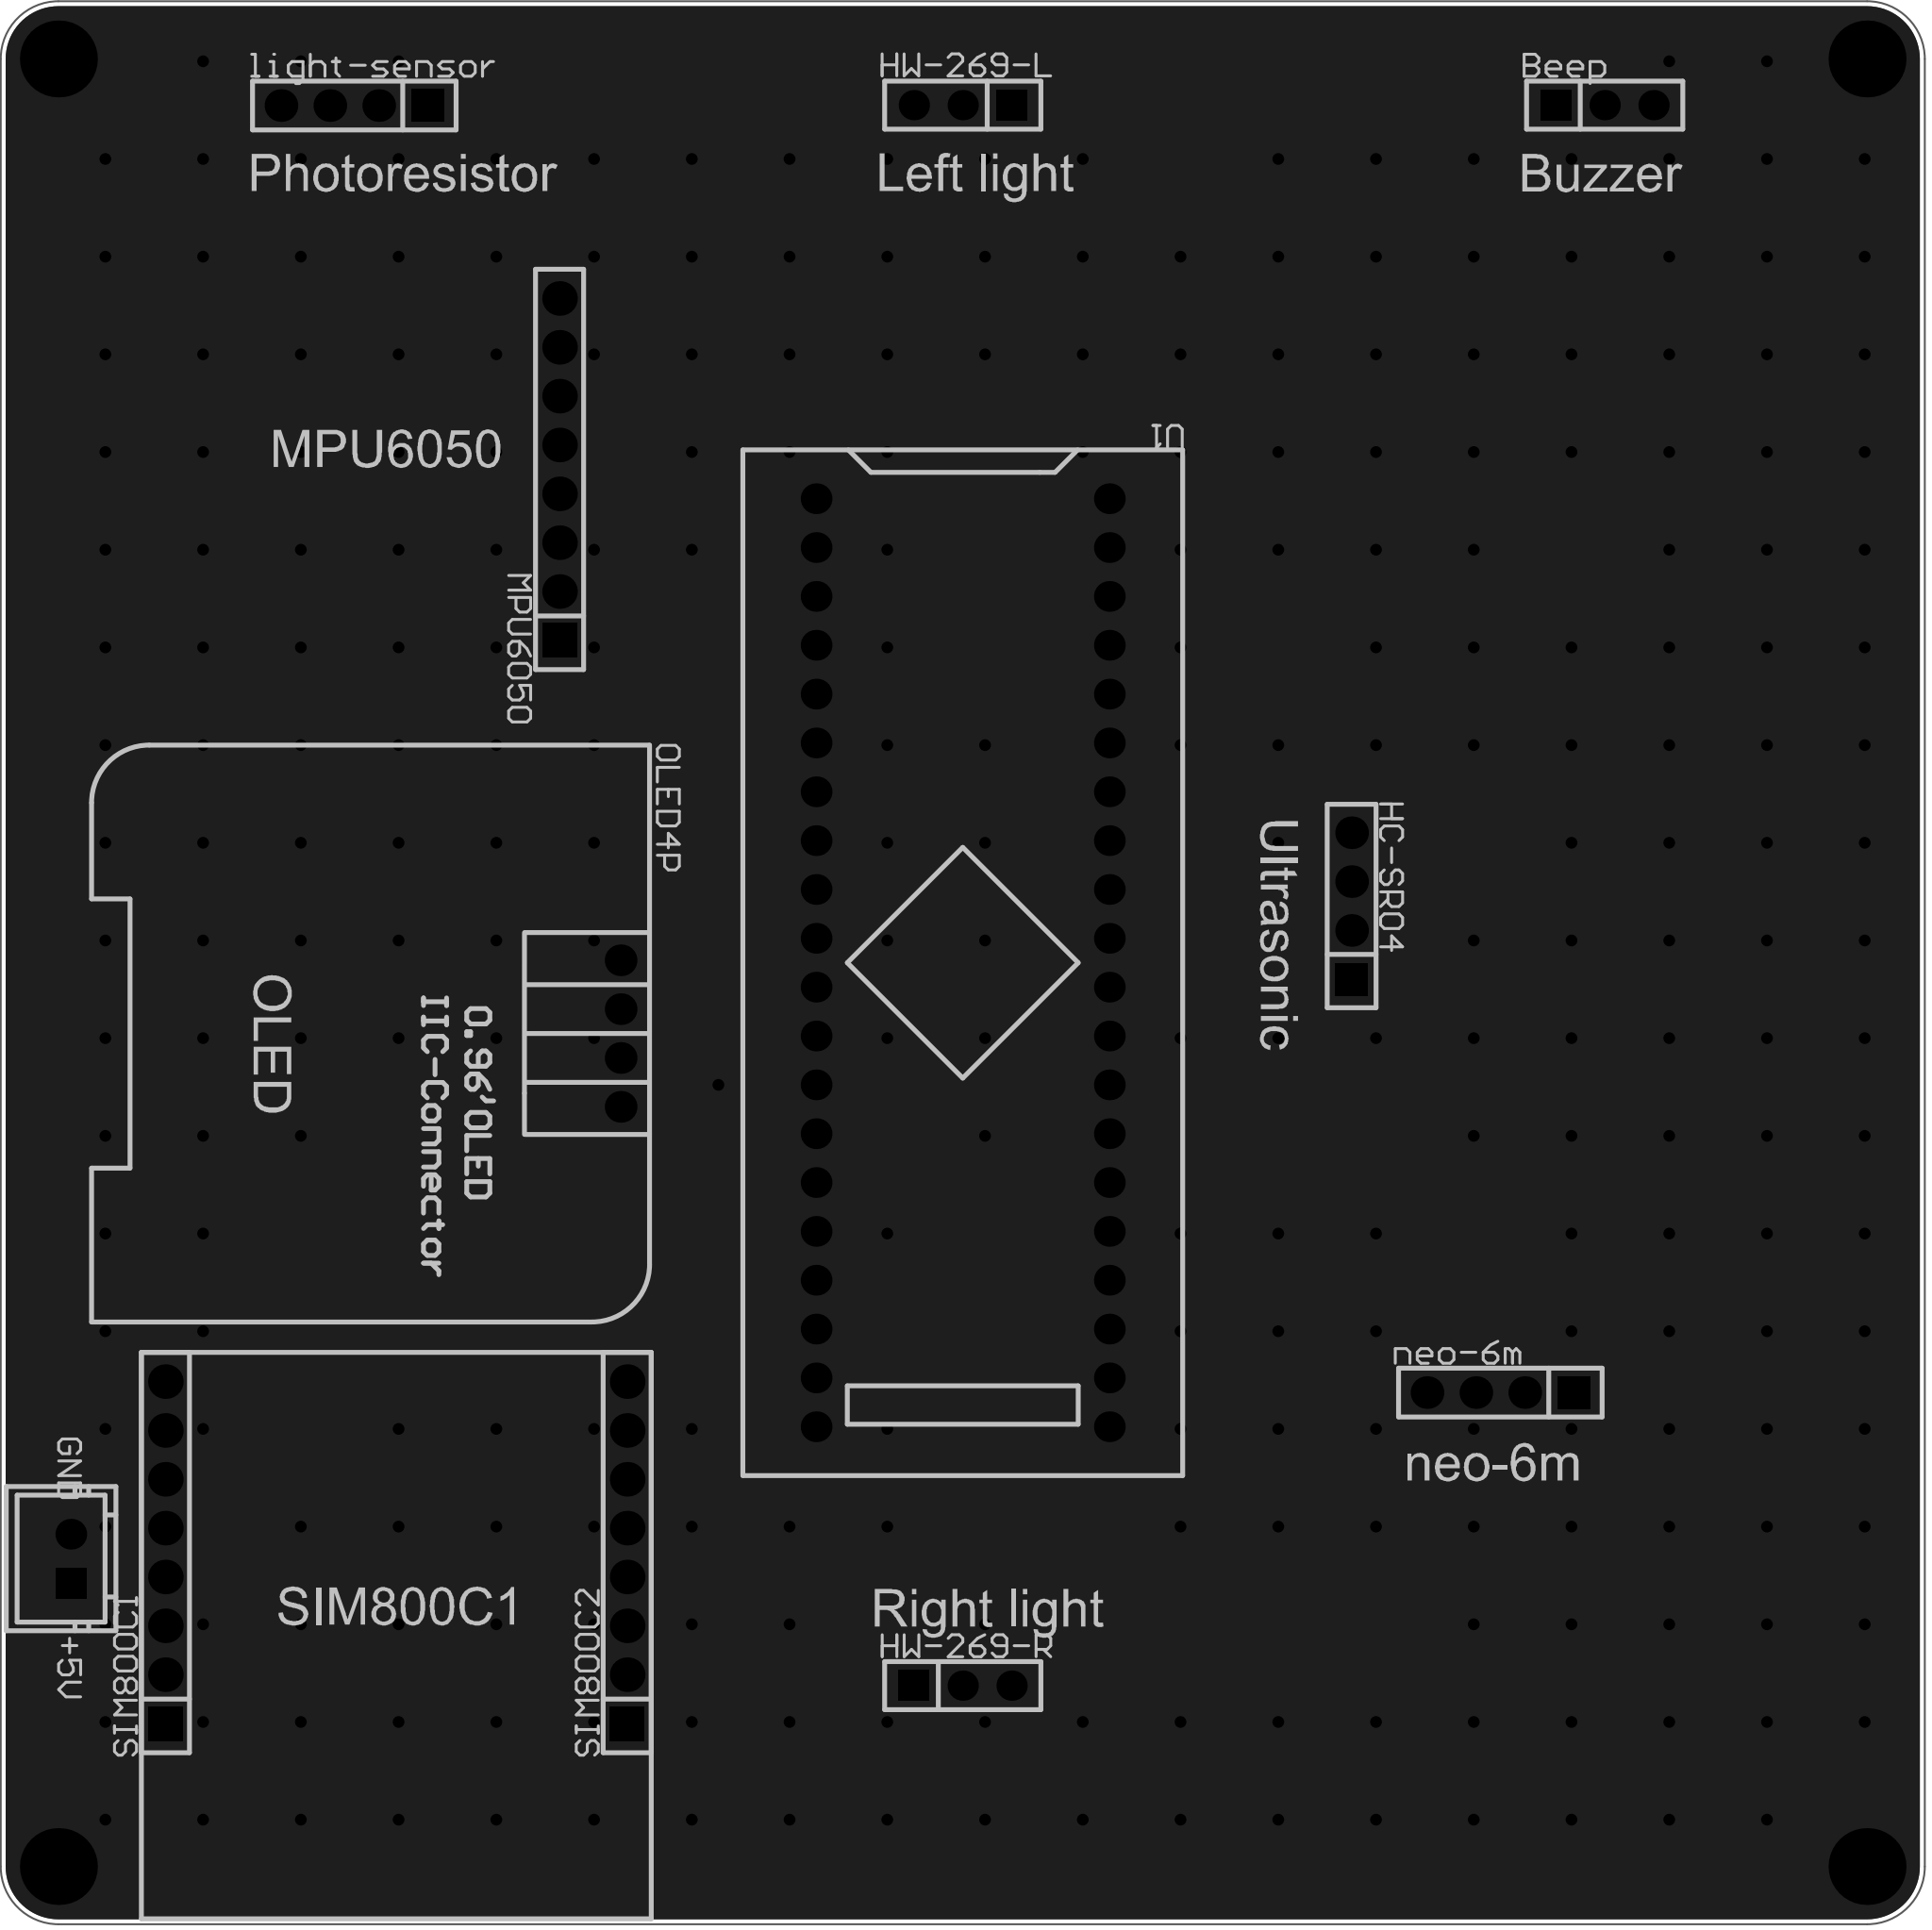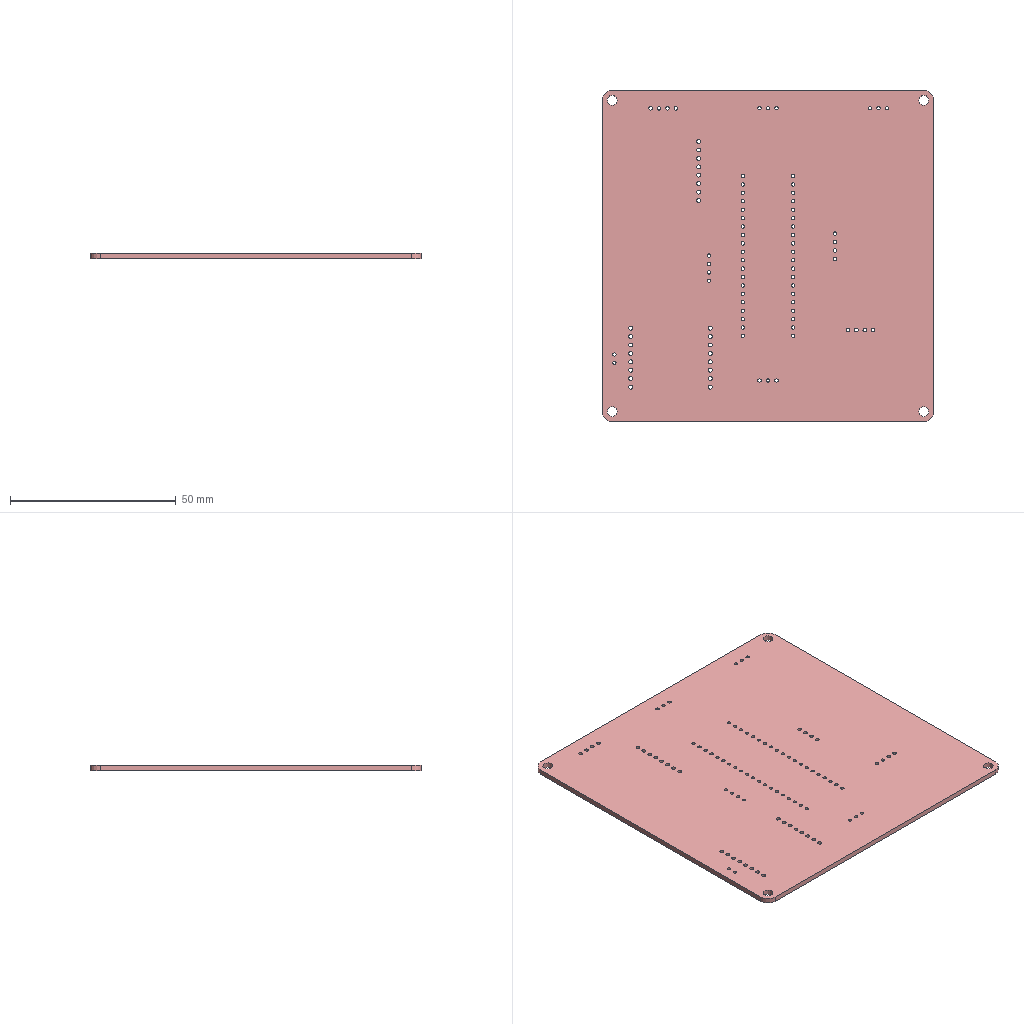Circuit board layout | Altium Designer | box 100 x 100 x 1.6 mm
Layer stack:
# Altium Designer layer stack of  (unit mm; dielectric type: 0 none, 1 core, 2 prepreg, 3 surface material)
index,name,kind,layer,copper_thickness_mm,dielectric_type,dielectric_thickness_mm,dielectric_material,dielectric_constant
0,Top Paste Mask Layer,other,,,,,,
1,Top Silkscreen Layer,other,,,,,,
2,Top Solder Mask Layer,dielectric,,,3,0.01,,3.3
3,Top Layer,copper,Top Layer,0.035,,,,
4,Dielectric1,dielectric,,,3,1.51,FR4,4.5
5,Bottom Layer,copper,Bottom Layer,0.035,,,,
6,Bottom Solder Mask Layer,dielectric,,,3,0.01,,3.3
7,Bottom Silkscreen Layer,other,,,,,,
8,Bottom Paste Mask Layer,other,,,,,,
# drill layer pairs: low layer,high layer
drill_pair,Top Layer,Bottom Layer
Part placement:
Designator,Comment,Layer,Footprint,Center-X(mm),Center-Y(mm),Rotation
U1,STM32F103C8T6-Card,TopLayer,CONN-TH_L53.3-W22.9_STM32F103C8T6-CARD,130.556,128.905,270
+5V,_x001F_XH2.54-2P,TopLayer,CONN-TH_2P-P2.54-V,84.201,97.917,90
OLED4P,,TopLayer,0.96OLED_4P,112.776,125.222,270
Beep,,TopLayer,HDR-TH_3P-P2.54-V-F,163.919,173.502,0
HC-SR04,,TopLayer,HDR-TH_4P-P2.54-V-F,150.767,131.855,90
HW-269-L,,TopLayer,HDR-TH_3P-P2.54-V-F,130.556,173.502,180
HW-269-R,,TopLayer,HDR-TH_3P-P2.54-V-F,130.556,91.313,0
light-sensor,,TopLayer,HDR-TH_4P-P2.54-V-F,98.933,173.482,180
neo-6m,,TopLayer,HDR-TH_4P-P2.54-V-F,158.496,106.553,180
MPU6050,,TopLayer,HDR-TH_8P-P2.54-V-F-1,109.601,154.559,90
SIM800C1,,TopLayer,HDR-TH_8P-P2.54-V-F-1,89.116,98.233,90
SIM800C2,,TopLayer,HDR-TH_8P-P2.54-V-F-1,113.116,98.233,90
Pad and via stacks:
# Altium Designer via and pad stacks of  (unit mm). Each distinct definition once, with the count of objects using it.
# via: kind,start_layer,end_layer,hole_mm,diameter_mm,mode(0 simple;1 top-mid-bottom;2 full stack),diameter_per_layer,count,example_net
# pad: kind,layer,hole_mm,hole_type(0 round;1 square;2 slot),plating,top_size,top_shape(1 round;2 rect;3 octagon;9 rounded rect),mid_size,bottom_size,mode,footprint,size_per_layer,count,example
pad,Multi-Layer,3,0,plated,4x4,1,4x4,4x4,0,,,4,1
pad,Multi-Layer,1,0,plated,1.6x1.6,1,1.6x1.6,1.6x1.6,0,CONN-TH_L53.3-W22.9_STM32F103C8T6-CARD,,40,U1.1
pad,Multi-Layer,1,0,plated,1.6x1.6,1,1.6x1.6,1.6x1.6,0,CONN-TH_2P-P2.54-V,,1,+5V.2
pad,Multi-Layer,1,0,plated,1.6x1.6,2,1.6x1.6,1.6x1.6,0,CONN-TH_2P-P2.54-V,,1,+5V.1
pad,Multi-Layer,1,0,plated,1.65x1.65,1,1.65x1.65,1.65x1.65,0,0.96OLED_4P,,4,OLED4P.4
pad,Multi-Layer,1.02,0,plated,1.575x1.575,1,1.575x1.575,1.575x1.575,0,HDR-TH_3P-P2.54-V-F,,6,Beep.3
pad,Multi-Layer,1.02,0,plated,1.575x1.575,2,1.575x1.575,1.575x1.575,0,HDR-TH_3P-P2.54-V-F,,3,Beep.1
pad,Multi-Layer,1.1,0,plated,1.7x1.7,2,1.7x1.7,1.7x1.7,0,HDR-TH_4P-P2.54-V-F,,3,HC-SR04.1
pad,Multi-Layer,1.1,0,plated,1.7x1.7,1,1.7x1.7,1.7x1.7,0,HDR-TH_4P-P2.54-V-F,,9,HC-SR04.2
pad,Multi-Layer,1.2,0,plated,1.8x1.8,2,1.8x1.8,1.8x1.8,0,HDR-TH_8P-P2.54-V-F-1,,3,MPU6050.1
pad,Multi-Layer,1.2,0,plated,1.8x1.8,1,1.8x1.8,1.8x1.8,0,HDR-TH_8P-P2.54-V-F-1,,21,MPU6050.2
via,Top Layer,Bottom Layer,0.3048,0.61,0,,276,PB5
Copper pours:
name,layer,net,type(0 solid;1 hatched;2 none)
Bottom Layer-GND,Bottom Layer,GND,0
Top Layer-GND,Top Layer,GND,0
Design rules, without the lines most boards share:
# Altium Designer design rules of  (exported by Altium Designer, unit mm)
# columns: name | kind | enabled | priority | scope1 | scope2 | descriptor | typed fields (field=value)
copperThickness1oz_2 | 2 | enabled | 2 | All | All | Width Constraint (Min=5mil) (Max=100mil) (Preferred=30mil) (All) |
viaSize | 11 | enabled | 1 | All | All | Routing Via (MinHoleWidth=11.811mil) (MaxHoleWidth=248.032mil) (PreferredHoleWidth=12.008mil) (MinWidth=19.685mil) (MaxWidth=393.701mil) (PreferedWidth=24.016mil) (All) | via_min_hole=0.3 via_max_hole=6.3 via_preferred_diameter=0.61 via_preferred_hole=0.305
solderMaskExpansion | 13 | enabled | 2 | All | All | Solder Mask Expansion (Expansion =2.008mil) (All) | expansion=0.051